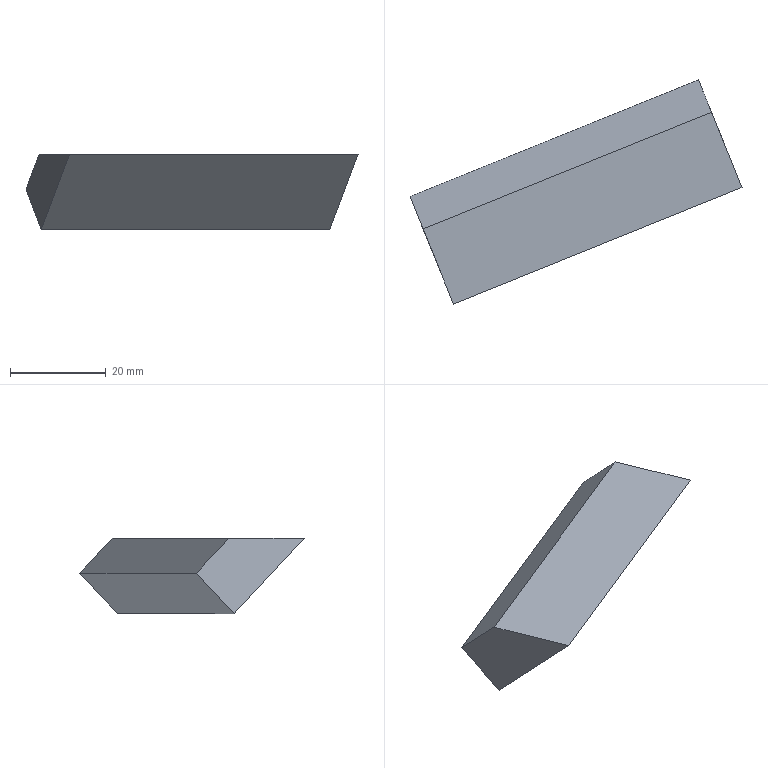Part | NX | features solid 2 | 1 solid | 6 faces | box 69.357 x 46.849 x 15.781 mm | volume 12728 mm3 | plane 6
STEP:
#1=CARTESIAN_POINT('',(-690.878,399.081,109.704));
#2=VERTEX_POINT('',#1);
#3=CARTESIAN_POINT('',(-688.145,392.316,117.));
#4=VERTEX_POINT('',#3);
#5=CARTESIAN_POINT('',(-692.895,404.072,104.321));
#6=DIRECTION('',(0.2649,-0.6556,0.7071));
#7=VECTOR('',#6,1000.);
#8=LINE('',#5,#7);
#9=EDGE_CURVE('',#2,#4,#8,.T.);
#10=ORIENTED_EDGE('',*,*,#9,.F.);
#11=CARTESIAN_POINT('',(-751.145,374.731,109.704));
#12=VERTEX_POINT('',#11);
#13=CARTESIAN_POINT('',(-751.145,374.731,109.704));
#14=DIRECTION('',(0.9272,0.3746,0.));
#15=VECTOR('',#14,1000.);
#16=LINE('',#13,#15);
#17=EDGE_CURVE('',#12,#2,#16,.T.);
#18=ORIENTED_EDGE('',*,*,#17,.F.);
#19=CARTESIAN_POINT('',(-748.412,367.967,117.));
#20=VERTEX_POINT('',#19);
#21=CARTESIAN_POINT('',(-753.162,379.722,104.321));
#22=DIRECTION('',(0.2649,-0.6556,0.7071));
#23=VECTOR('',#22,1000.);
#24=LINE('',#21,#23);
#25=EDGE_CURVE('',#12,#20,#24,.T.);
#26=ORIENTED_EDGE('',*,*,#25,.T.);
#27=CARTESIAN_POINT('',(-688.145,392.316,117.));
#28=DIRECTION('',(0.9272,0.3746,0.));
#29=VECTOR('',#28,1000.);
#30=LINE('',#27,#29);
#31=EDGE_CURVE('',#20,#4,#30,.T.);
#32=ORIENTED_EDGE('',*,*,#31,.T.);
#33=EDGE_LOOP('',(#10,#18,#26,#32));
#34=FACE_BOUND('',#33,.T.);
#35=CARTESIAN_POINT('',(-753.162,379.722,104.321));
#36=DIRECTION('',(0.2649,-0.6556,-0.7071));
#37=DIRECTION('',(0.2649,-0.6556,0.7071));
#38=AXIS2_PLACEMENT_3D('',#35,#36,#37);
#39=PLANE('',#38);
#40=ADVANCED_FACE('',(#34),#39,.F.);
#41=CARTESIAN_POINT('',(-681.788,376.581,117.));
#42=VERTEX_POINT('',#41);
#43=CARTESIAN_POINT('',(-709.026,443.998,117.));
#44=DIRECTION('',(0.3746,-0.9272,0.));
#45=VECTOR('',#44,1000.);
#46=LINE('',#43,#45);
#47=EDGE_CURVE('',#4,#42,#46,.T.);
#48=ORIENTED_EDGE('',*,*,#47,.F.);
#49=ORIENTED_EDGE('',*,*,#31,.F.);
#50=CARTESIAN_POINT('',(-742.055,352.232,117.));
#51=VERTEX_POINT('',#50);
#52=CARTESIAN_POINT('',(-769.293,419.648,117.));
#53=DIRECTION('',(0.3746,-0.9272,0.));
#54=VECTOR('',#53,1000.);
#55=LINE('',#52,#54);
#56=EDGE_CURVE('',#20,#51,#55,.T.);
#57=ORIENTED_EDGE('',*,*,#56,.T.);
#58=CARTESIAN_POINT('',(-681.788,376.581,117.));
#59=DIRECTION('',(0.9272,0.3746,0.));
#60=VECTOR('',#59,1000.);
#61=LINE('',#58,#60);
#62=EDGE_CURVE('',#51,#42,#61,.T.);
#63=ORIENTED_EDGE('',*,*,#62,.T.);
#64=EDGE_LOOP('',(#48,#49,#57,#63));
#65=FACE_BOUND('',#64,.T.);
#66=CARTESIAN_POINT('',(-709.026,443.998,117.));
#67=DIRECTION('',(0.,0.,-1.));
#68=DIRECTION('',(0.3746,-0.9272,0.));
#69=AXIS2_PLACEMENT_3D('',#66,#67,#68);
#70=PLANE('',#69);
#71=ADVANCED_FACE('',(#65),#70,.F.);
#72=CARTESIAN_POINT('',(-687.7,391.213,101.219));
#73=VERTEX_POINT('',#72);
#74=CARTESIAN_POINT('',(-689.716,396.204,95.836));
#75=DIRECTION('',(0.2649,-0.6556,0.7071));
#76=VECTOR('',#75,1000.);
#77=LINE('',#74,#76);
#78=EDGE_CURVE('',#73,#42,#77,.T.);
#79=ORIENTED_EDGE('',*,*,#78,.T.);
#80=ORIENTED_EDGE('',*,*,#62,.F.);
#81=CARTESIAN_POINT('',(-747.967,366.864,101.219));
#82=VERTEX_POINT('',#81);
#83=CARTESIAN_POINT('',(-749.983,371.855,95.836));
#84=DIRECTION('',(0.2649,-0.6556,0.7071));
#85=VECTOR('',#84,1000.);
#86=LINE('',#83,#85);
#87=EDGE_CURVE('',#82,#51,#86,.T.);
#88=ORIENTED_EDGE('',*,*,#87,.F.);
#89=CARTESIAN_POINT('',(-747.967,366.864,101.219));
#90=DIRECTION('',(0.9272,0.3746,0.));
#91=VECTOR('',#90,1000.);
#92=LINE('',#89,#91);
#93=EDGE_CURVE('',#82,#73,#92,.T.);
#94=ORIENTED_EDGE('',*,*,#93,.T.);
#95=EDGE_LOOP('',(#79,#80,#88,#94));
#96=FACE_BOUND('',#95,.T.);
#97=CARTESIAN_POINT('',(-749.983,371.855,95.836));
#98=DIRECTION('',(0.2649,-0.6556,-0.7071));
#99=DIRECTION('',(0.2649,-0.6556,0.7071));
#100=AXIS2_PLACEMENT_3D('',#97,#98,#99);
#101=PLANE('',#100);
#102=ADVANCED_FACE('',(#96),#101,.T.);
#103=CARTESIAN_POINT('',(-690.878,399.081,109.704));
#104=DIRECTION('',(0.2649,-0.6556,-0.7071));
#105=VECTOR('',#104,1000.);
#106=LINE('',#103,#105);
#107=EDGE_CURVE('',#2,#73,#106,.T.);
#108=ORIENTED_EDGE('',*,*,#107,.T.);
#109=ORIENTED_EDGE('',*,*,#93,.F.);
#110=CARTESIAN_POINT('',(-751.145,374.731,109.704));
#111=DIRECTION('',(0.2649,-0.6556,-0.7071));
#112=VECTOR('',#111,1000.);
#113=LINE('',#110,#112);
#114=EDGE_CURVE('',#12,#82,#113,.T.);
#115=ORIENTED_EDGE('',*,*,#114,.F.);
#116=ORIENTED_EDGE('',*,*,#17,.T.);
#117=EDGE_LOOP('',(#108,#109,#115,#116));
#118=FACE_BOUND('',#117,.T.);
#119=CARTESIAN_POINT('',(-751.145,374.731,109.704));
#120=DIRECTION('',(-0.2649,0.6556,-0.7071));
#121=DIRECTION('',(0.2649,-0.6556,-0.7071));
#122=AXIS2_PLACEMENT_3D('',#119,#120,#121);
#123=PLANE('',#122);
#124=ADVANCED_FACE('',(#118),#123,.T.);
#125=ORIENTED_EDGE('',*,*,#25,.F.);
#126=ORIENTED_EDGE('',*,*,#114,.T.);
#127=ORIENTED_EDGE('',*,*,#87,.T.);
#128=ORIENTED_EDGE('',*,*,#56,.F.);
#129=EDGE_LOOP('',(#125,#126,#127,#128));
#130=FACE_BOUND('',#129,.T.);
#131=CARTESIAN_POINT('',(-753.162,379.722,104.321));
#132=DIRECTION('',(-0.9272,-0.3746,0.));
#133=DIRECTION('',(-0.352,0.8713,-0.342));
#134=AXIS2_PLACEMENT_3D('',#131,#132,#133);
#135=PLANE('',#134);
#136=ADVANCED_FACE('',(#130),#135,.T.);
#137=ORIENTED_EDGE('',*,*,#9,.T.);
#138=ORIENTED_EDGE('',*,*,#47,.T.);
#139=ORIENTED_EDGE('',*,*,#78,.F.);
#140=ORIENTED_EDGE('',*,*,#107,.F.);
#141=EDGE_LOOP('',(#137,#138,#139,#140));
#142=FACE_BOUND('',#141,.T.);
#143=CARTESIAN_POINT('',(-692.895,404.072,104.321));
#144=DIRECTION('',(-0.9272,-0.3746,0.));
#145=DIRECTION('',(-0.352,0.8713,-0.342));
#146=AXIS2_PLACEMENT_3D('',#143,#144,#145);
#147=PLANE('',#146);
#148=ADVANCED_FACE('',(#142),#147,.F.);
#149=CLOSED_SHELL('',(#40,#71,#102,#124,#136,#148));
#150=MANIFOLD_SOLID_BREP('',#149);
#151=(LENGTH_UNIT()NAMED_UNIT(*)SI_UNIT(.MILLI.,.METRE.));
#152=UNCERTAINTY_MEASURE_WITH_UNIT(LENGTH_MEASURE(0.00001),#151,'','');
#153=(NAMED_UNIT(*)PLANE_ANGLE_UNIT()SI_UNIT($,.RADIAN.));
#154=(NAMED_UNIT(*)SI_UNIT($,.STERADIAN.)SOLID_ANGLE_UNIT());
#155=(GEOMETRIC_REPRESENTATION_CONTEXT(3)GLOBAL_UNCERTAINTY_ASSIGNED_CONTEXT((#152))GLOBAL_UNIT_ASSIGNED_CONTEXT((#151,#153,#154))REPRESENTATION_CONTEXT('',''));
#156=ADVANCED_BREP_SHAPE_REPRESENTATION('',(#150),#155);